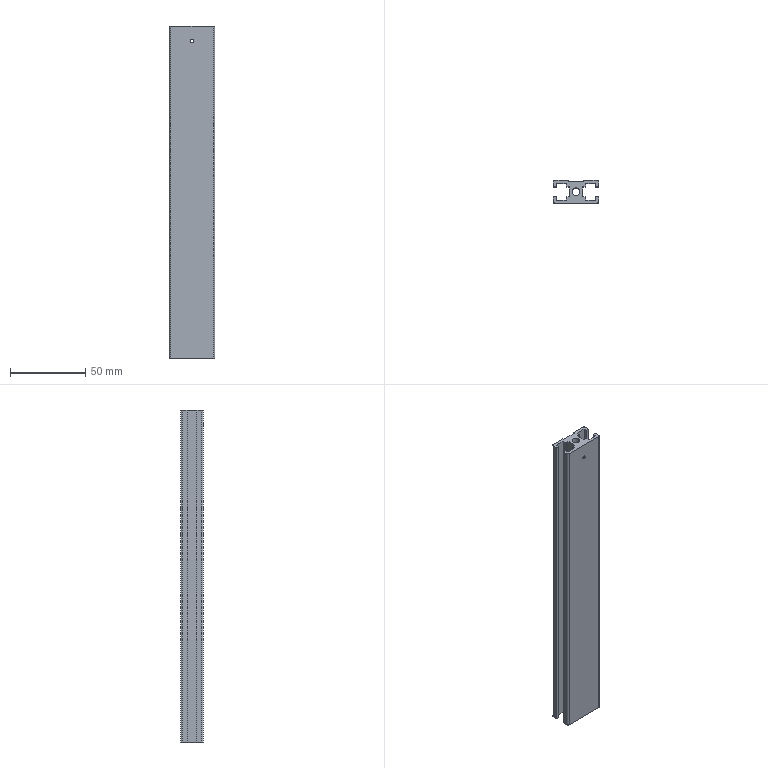Part | 1 solid | 72 faces | box 30 x 15 x 220 mm | volume 49022 mm3 | plane 42 | cylinder 30 | commonest cylinder face diameters 3.2 x16 1 x4 2 x4 2.2 x4 5.1 x2